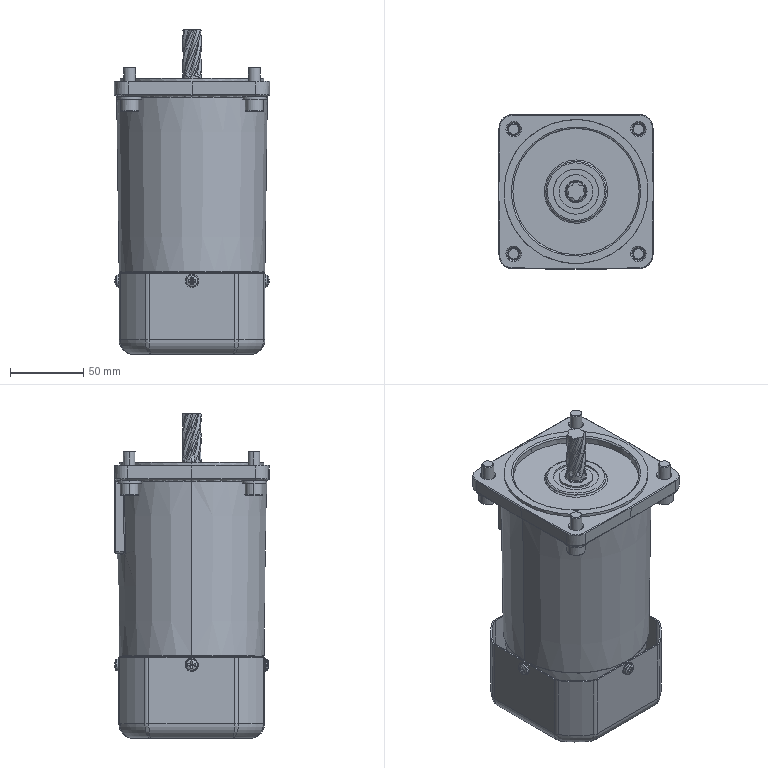Part | STEP file | 11-100YB200G11 | 2 solids | 749 faces | box 105.972 x 105.485 x 221 mm | volume 385712 mm3 | cylinder 291 | plane 191 | spline 113 | torus 89 | cone 43 | sphere 22 | commonest cylinder face diameters 3 x54 4 x42 1 x24 8 x24 0.4 x16 1.6 x11